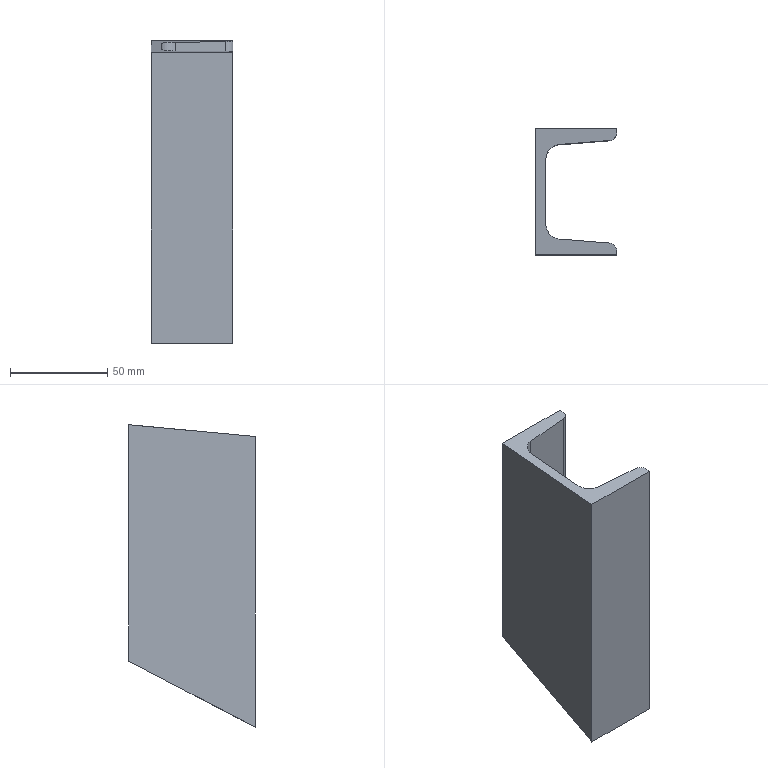Part | STEP file | DIN 1026-1 U 65 1785415623083 | 1 solid | 14 faces | box 42 x 65 x 155.66 mm | volume 122460 mm3 | plane 10 | cylinder 4 | commonest cylinder face diameters 8 x2 15 x2
STEP:
#1=CARTESIAN_POINT('',(42.,30.373,-1.115));
#2=VERTEX_POINT('',#1);
#3=CARTESIAN_POINT('',(42.,32.5,0.));
#4=VERTEX_POINT('',#3);
#5=CARTESIAN_POINT('',(42.,19.754,-6.683));
#6=DIRECTION('',(0.,0.8857,0.4643));
#7=VECTOR('',#6,10.);
#8=LINE('',#5,#7);
#9=EDGE_CURVE('',#2,#4,#8,.T.);
#10=ORIENTED_EDGE('',*,*,#9,.F.);
#11=CARTESIAN_POINT('',(38.319,26.386,-3.206));
#12=VERTEX_POINT('',#11);
#13=CARTESIAN_POINT('',(38.,30.373,-1.115));
#14=DIRECTION('',(0.,-0.4643,0.8857));
#15=DIRECTION('',(0.,0.8857,0.4643));
#16=AXIS2_PLACEMENT_3D('',#13,#14,#15);
#17=ELLIPSE('',#16,4.516,4.);
#18=EDGE_CURVE('',#12,#2,#17,.T.);
#19=ORIENTED_EDGE('',*,*,#18,.F.);
#20=CARTESIAN_POINT('',(12.402,24.312,-4.293));
#21=VERTEX_POINT('',#20);
#22=CARTESIAN_POINT('',(18.401,24.792,-4.041));
#23=DIRECTION('',(0.9959,0.07968,0.04177));
#24=VECTOR('',#23,10.);
#25=LINE('',#22,#24);
#26=EDGE_CURVE('',#21,#12,#25,.T.);
#27=ORIENTED_EDGE('',*,*,#26,.F.);
#28=CARTESIAN_POINT('',(5.5,16.836,-8.212));
#29=VERTEX_POINT('',#28);
#30=CARTESIAN_POINT('',(13.,16.836,-8.212));
#31=DIRECTION('',(0.,0.4643,-0.8857));
#32=DIRECTION('',(0.,0.8857,0.4643));
#33=AXIS2_PLACEMENT_3D('',#30,#31,#32);
#34=ELLIPSE('',#33,8.468,7.5);
#35=EDGE_CURVE('',#29,#21,#34,.T.);
#36=ORIENTED_EDGE('',*,*,#35,.F.);
#37=CARTESIAN_POINT('',(5.5,-16.836,-25.866));
#38=VERTEX_POINT('',#37);
#39=CARTESIAN_POINT('',(5.5,7.007,-13.365));
#40=DIRECTION('',(0.,0.8857,0.4643));
#41=VECTOR('',#40,10.);
#42=LINE('',#39,#41);
#43=EDGE_CURVE('',#38,#29,#42,.T.);
#44=ORIENTED_EDGE('',*,*,#43,.F.);
#45=CARTESIAN_POINT('',(12.402,-24.312,-29.786));
#46=VERTEX_POINT('',#45);
#47=CARTESIAN_POINT('',(13.,-16.836,-25.866));
#48=DIRECTION('',(0.,0.4643,-0.8857));
#49=DIRECTION('',(0.,-0.8857,-0.4643));
#50=AXIS2_PLACEMENT_3D('',#47,#48,#49);
#51=ELLIPSE('',#50,8.468,7.5);
#52=EDGE_CURVE('',#46,#38,#51,.T.);
#53=ORIENTED_EDGE('',*,*,#52,.F.);
#54=CARTESIAN_POINT('',(38.319,-26.386,-30.873));
#55=VERTEX_POINT('',#54);
#56=CARTESIAN_POINT('',(4.047,-23.644,-29.436));
#57=DIRECTION('',(-0.9959,0.07968,0.04177));
#58=VECTOR('',#57,10.);
#59=LINE('',#56,#58);
#60=EDGE_CURVE('',#55,#46,#59,.T.);
#61=ORIENTED_EDGE('',*,*,#60,.F.);
#62=CARTESIAN_POINT('',(42.,-30.373,-32.963));
#63=VERTEX_POINT('',#62);
#64=CARTESIAN_POINT('',(38.,-30.373,-32.963));
#65=DIRECTION('',(0.,-0.4643,0.8857));
#66=DIRECTION('',(0.,-0.8857,-0.4643));
#67=AXIS2_PLACEMENT_3D('',#64,#65,#66);
#68=ELLIPSE('',#67,4.516,4.);
#69=EDGE_CURVE('',#63,#55,#68,.T.);
#70=ORIENTED_EDGE('',*,*,#69,.F.);
#71=CARTESIAN_POINT('',(42.,-32.5,-34.079));
#72=VERTEX_POINT('',#71);
#73=CARTESIAN_POINT('',(42.,-4.905,-19.611));
#74=DIRECTION('',(0.,0.8857,0.4643));
#75=VECTOR('',#74,10.);
#76=LINE('',#73,#75);
#77=EDGE_CURVE('',#72,#63,#76,.T.);
#78=ORIENTED_EDGE('',*,*,#77,.F.);
#79=CARTESIAN_POINT('',(0.,-32.5,-34.079));
#80=VERTEX_POINT('',#79);
#81=CARTESIAN_POINT('',(31.5,-32.5,-34.079));
#82=DIRECTION('',(-1.,0.,0.));
#83=VECTOR('',#82,10.);
#84=LINE('',#81,#83);
#85=EDGE_CURVE('',#72,#80,#84,.T.);
#86=ORIENTED_EDGE('',*,*,#85,.T.);
#87=CARTESIAN_POINT('',(0.,32.5,0.));
#88=VERTEX_POINT('',#87);
#89=CARTESIAN_POINT('',(0.,7.007,-13.365));
#90=DIRECTION('',(0.,-0.8857,-0.4643));
#91=VECTOR('',#90,10.);
#92=LINE('',#89,#91);
#93=EDGE_CURVE('',#88,#80,#92,.T.);
#94=ORIENTED_EDGE('',*,*,#93,.F.);
#95=CARTESIAN_POINT('',(0.,32.5,0.));
#96=DIRECTION('',(-1.,0.,0.));
#97=VECTOR('',#96,10.);
#98=LINE('',#95,#97);
#99=EDGE_CURVE('',#4,#88,#98,.T.);
#100=ORIENTED_EDGE('',*,*,#99,.F.);
#101=EDGE_LOOP('',(#10,#19,#27,#36,#44,#53,#61,#70,#78,#86,#94,#100));
#102=FACE_OUTER_BOUND('',#101,.T.);
#103=CARTESIAN_POINT('',(0.,7.007,-13.365));
#104=DIRECTION('',(0.,-0.4643,0.8857));
#105=DIRECTION('',(1.,0.,0.));
#106=AXIS2_PLACEMENT_3D('',#103,#104,#105);
#107=PLANE('',#106);
#108=ADVANCED_FACE('',(#102),#107,.F.);
#109=ORIENTED_EDGE('',*,*,#60,.T.);
#110=CARTESIAN_POINT('',(12.402,-24.312,116.262));
#111=VERTEX_POINT('',#110);
#112=CARTESIAN_POINT('',(12.402,-24.312,0.));
#113=DIRECTION('',(0.,0.,-1.));
#114=VECTOR('',#113,10.);
#115=LINE('',#112,#114);
#116=EDGE_CURVE('',#111,#46,#115,.T.);
#117=ORIENTED_EDGE('',*,*,#116,.F.);
#118=CARTESIAN_POINT('',(38.319,-26.386,116.068));
#119=VERTEX_POINT('',#118);
#120=CARTESIAN_POINT('',(6.14,-23.811,116.309));
#121=DIRECTION('',(0.9968,-0.07974,-0.007467));
#122=VECTOR('',#121,10.);
#123=LINE('',#120,#122);
#124=EDGE_CURVE('',#111,#119,#123,.T.);
#125=ORIENTED_EDGE('',*,*,#124,.T.);
#126=CARTESIAN_POINT('',(38.319,-26.386,0.));
#127=DIRECTION('',(0.,0.,-1.));
#128=VECTOR('',#127,10.);
#129=LINE('',#126,#128);
#130=EDGE_CURVE('',#119,#55,#129,.T.);
#131=ORIENTED_EDGE('',*,*,#130,.T.);
#132=EDGE_LOOP('',(#109,#117,#125,#131));
#133=FACE_OUTER_BOUND('',#132,.T.);
#134=CARTESIAN_POINT('',(12.402,-24.312,0.));
#135=DIRECTION('',(0.07975,0.9968,0.));
#136=DIRECTION('',(0.,0.,1.));
#137=AXIS2_PLACEMENT_3D('',#134,#135,#136);
#138=PLANE('',#137);
#139=ADVANCED_FACE('',(#133),#138,.T.);
#140=ORIENTED_EDGE('',*,*,#52,.T.);
#141=CARTESIAN_POINT('',(5.5,-16.836,116.962));
#142=VERTEX_POINT('',#141);
#143=CARTESIAN_POINT('',(5.5,-16.836,0.));
#144=DIRECTION('',(0.,0.,-1.));
#145=VECTOR('',#144,10.);
#146=LINE('',#143,#145);
#147=EDGE_CURVE('',#142,#38,#146,.T.);
#148=ORIENTED_EDGE('',*,*,#147,.F.);
#149=CARTESIAN_POINT('',(13.,-16.836,116.962));
#150=DIRECTION('',(0.,-0.09323,0.9956));
#151=DIRECTION('',(0.,-0.9956,-0.09323));
#152=AXIS2_PLACEMENT_3D('',#149,#150,#151);
#153=ELLIPSE('',#152,7.533,7.5);
#154=EDGE_CURVE('',#142,#111,#153,.T.);
#155=ORIENTED_EDGE('',*,*,#154,.T.);
#156=ORIENTED_EDGE('',*,*,#116,.T.);
#157=EDGE_LOOP('',(#140,#148,#155,#156));
#158=FACE_OUTER_BOUND('',#157,.T.);
#159=CARTESIAN_POINT('',(13.,-16.836,0.));
#160=DIRECTION('',(0.,0.,1.));
#161=DIRECTION('',(-1.,0.,0.));
#162=AXIS2_PLACEMENT_3D('',#159,#160,#161);
#163=CYLINDRICAL_SURFACE('',#162,7.5);
#164=ADVANCED_FACE('',(#158),#163,.F.);
#165=ORIENTED_EDGE('',*,*,#43,.T.);
#166=CARTESIAN_POINT('',(5.5,16.836,120.115));
#167=VERTEX_POINT('',#166);
#168=CARTESIAN_POINT('',(5.5,16.836,0.));
#169=DIRECTION('',(0.,0.,-1.));
#170=VECTOR('',#169,10.);
#171=LINE('',#168,#170);
#172=EDGE_CURVE('',#167,#29,#171,.T.);
#173=ORIENTED_EDGE('',*,*,#172,.F.);
#174=CARTESIAN_POINT('',(5.5,-11.004,117.508));
#175=DIRECTION('',(0.,-0.9956,-0.09323));
#176=VECTOR('',#175,10.);
#177=LINE('',#174,#176);
#178=EDGE_CURVE('',#167,#142,#177,.T.);
#179=ORIENTED_EDGE('',*,*,#178,.T.);
#180=ORIENTED_EDGE('',*,*,#147,.T.);
#181=EDGE_LOOP('',(#165,#173,#179,#180));
#182=FACE_OUTER_BOUND('',#181,.T.);
#183=CARTESIAN_POINT('',(5.5,0.,0.));
#184=DIRECTION('',(1.,0.,0.));
#185=DIRECTION('',(0.,0.,-1.));
#186=AXIS2_PLACEMENT_3D('',#183,#184,#185);
#187=PLANE('',#186);
#188=ADVANCED_FACE('',(#182),#187,.T.);
#189=ORIENTED_EDGE('',*,*,#35,.T.);
#190=CARTESIAN_POINT('',(12.402,24.312,120.815));
#191=VERTEX_POINT('',#190);
#192=CARTESIAN_POINT('',(12.402,24.312,0.));
#193=DIRECTION('',(0.,0.,-1.));
#194=VECTOR('',#193,10.);
#195=LINE('',#192,#194);
#196=EDGE_CURVE('',#191,#21,#195,.T.);
#197=ORIENTED_EDGE('',*,*,#196,.F.);
#198=CARTESIAN_POINT('',(13.,16.836,120.115));
#199=DIRECTION('',(0.,-0.09323,0.9956));
#200=DIRECTION('',(0.,0.9956,0.09323));
#201=AXIS2_PLACEMENT_3D('',#198,#199,#200);
#202=ELLIPSE('',#201,7.533,7.5);
#203=EDGE_CURVE('',#191,#167,#202,.T.);
#204=ORIENTED_EDGE('',*,*,#203,.T.);
#205=ORIENTED_EDGE('',*,*,#172,.T.);
#206=EDGE_LOOP('',(#189,#197,#204,#205));
#207=FACE_OUTER_BOUND('',#206,.T.);
#208=CARTESIAN_POINT('',(13.,16.836,0.));
#209=DIRECTION('',(0.,0.,1.));
#210=DIRECTION('',(-0.07975,0.9968,0.));
#211=AXIS2_PLACEMENT_3D('',#208,#209,#210);
#212=CYLINDRICAL_SURFACE('',#211,7.5);
#213=ADVANCED_FACE('',(#207),#212,.F.);
#214=ORIENTED_EDGE('',*,*,#26,.T.);
#215=CARTESIAN_POINT('',(38.319,26.386,121.009));
#216=VERTEX_POINT('',#215);
#217=CARTESIAN_POINT('',(38.319,26.386,0.));
#218=DIRECTION('',(0.,0.,-1.));
#219=VECTOR('',#218,10.);
#220=LINE('',#217,#219);
#221=EDGE_CURVE('',#216,#12,#220,.T.);
#222=ORIENTED_EDGE('',*,*,#221,.F.);
#223=CARTESIAN_POINT('',(17.333,24.707,120.852));
#224=DIRECTION('',(-0.9968,-0.07974,-0.007467));
#225=VECTOR('',#224,10.);
#226=LINE('',#223,#225);
#227=EDGE_CURVE('',#216,#191,#226,.T.);
#228=ORIENTED_EDGE('',*,*,#227,.T.);
#229=ORIENTED_EDGE('',*,*,#196,.T.);
#230=EDGE_LOOP('',(#214,#222,#228,#229));
#231=FACE_OUTER_BOUND('',#230,.T.);
#232=CARTESIAN_POINT('',(38.319,26.386,0.));
#233=DIRECTION('',(0.07975,-0.9968,0.));
#234=DIRECTION('',(0.,0.,-1.));
#235=AXIS2_PLACEMENT_3D('',#232,#233,#234);
#236=PLANE('',#235);
#237=ADVANCED_FACE('',(#231),#236,.T.);
#238=ORIENTED_EDGE('',*,*,#18,.T.);
#239=CARTESIAN_POINT('',(42.,30.373,121.383));
#240=VERTEX_POINT('',#239);
#241=CARTESIAN_POINT('',(42.,30.373,0.));
#242=DIRECTION('',(0.,0.,-1.));
#243=VECTOR('',#242,10.);
#244=LINE('',#241,#243);
#245=EDGE_CURVE('',#240,#2,#244,.T.);
#246=ORIENTED_EDGE('',*,*,#245,.F.);
#247=CARTESIAN_POINT('',(38.,30.373,121.383));
#248=DIRECTION('',(0.,0.09323,-0.9956));
#249=DIRECTION('',(0.,0.9956,0.09323));
#250=AXIS2_PLACEMENT_3D('',#247,#248,#249);
#251=ELLIPSE('',#250,4.017,4.);
#252=EDGE_CURVE('',#240,#216,#251,.T.);
#253=ORIENTED_EDGE('',*,*,#252,.T.);
#254=ORIENTED_EDGE('',*,*,#221,.T.);
#255=EDGE_LOOP('',(#238,#246,#253,#254));
#256=FACE_OUTER_BOUND('',#255,.T.);
#257=CARTESIAN_POINT('',(38.,30.373,0.));
#258=DIRECTION('',(0.,0.,1.));
#259=DIRECTION('',(-0.07975,0.9968,0.));
#260=AXIS2_PLACEMENT_3D('',#257,#258,#259);
#261=CYLINDRICAL_SURFACE('',#260,4.);
#262=ADVANCED_FACE('',(#256),#261,.T.);
#263=ORIENTED_EDGE('',*,*,#154,.F.);
#264=ORIENTED_EDGE('',*,*,#178,.F.);
#265=ORIENTED_EDGE('',*,*,#203,.F.);
#266=ORIENTED_EDGE('',*,*,#227,.F.);
#267=ORIENTED_EDGE('',*,*,#252,.F.);
#268=CARTESIAN_POINT('',(42.,32.5,121.582));
#269=VERTEX_POINT('',#268);
#270=CARTESIAN_POINT('',(42.,5.105,119.016));
#271=DIRECTION('',(0.,-0.9956,-0.09323));
#272=VECTOR('',#271,10.);
#273=LINE('',#270,#272);
#274=EDGE_CURVE('',#269,#240,#273,.T.);
#275=ORIENTED_EDGE('',*,*,#274,.F.);
#276=CARTESIAN_POINT('',(0.,32.5,121.582));
#277=VERTEX_POINT('',#276);
#278=CARTESIAN_POINT('',(10.5,32.5,121.582));
#279=DIRECTION('',(1.,0.,0.));
#280=VECTOR('',#279,10.);
#281=LINE('',#278,#280);
#282=EDGE_CURVE('',#277,#269,#281,.T.);
#283=ORIENTED_EDGE('',*,*,#282,.F.);
#284=CARTESIAN_POINT('',(0.,-32.5,115.495));
#285=VERTEX_POINT('',#284);
#286=CARTESIAN_POINT('',(0.,-11.004,117.508));
#287=DIRECTION('',(0.,0.9956,0.09323));
#288=VECTOR('',#287,10.);
#289=LINE('',#286,#288);
#290=EDGE_CURVE('',#285,#277,#289,.T.);
#291=ORIENTED_EDGE('',*,*,#290,.F.);
#292=CARTESIAN_POINT('',(42.,-32.5,115.495));
#293=VERTEX_POINT('',#292);
#294=CARTESIAN_POINT('',(21.,-32.5,115.495));
#295=DIRECTION('',(-1.,0.,0.));
#296=VECTOR('',#295,10.);
#297=LINE('',#294,#296);
#298=EDGE_CURVE('',#293,#285,#297,.T.);
#299=ORIENTED_EDGE('',*,*,#298,.F.);
#300=CARTESIAN_POINT('',(42.,-30.373,115.694));
#301=VERTEX_POINT('',#300);
#302=CARTESIAN_POINT('',(42.,-26.058,116.098));
#303=DIRECTION('',(0.,-0.9956,-0.09323));
#304=VECTOR('',#303,10.);
#305=LINE('',#302,#304);
#306=EDGE_CURVE('',#301,#293,#305,.T.);
#307=ORIENTED_EDGE('',*,*,#306,.F.);
#308=CARTESIAN_POINT('',(38.,-30.373,115.694));
#309=DIRECTION('',(0.,0.09323,-0.9956));
#310=DIRECTION('',(0.,-0.9956,-0.09323));
#311=AXIS2_PLACEMENT_3D('',#308,#309,#310);
#312=ELLIPSE('',#311,4.017,4.);
#313=EDGE_CURVE('',#119,#301,#312,.T.);
#314=ORIENTED_EDGE('',*,*,#313,.F.);
#315=ORIENTED_EDGE('',*,*,#124,.F.);
#316=EDGE_LOOP('',(#263,#264,#265,#266,#267,#275,#283,#291,#299,#307,#314,#315));
#317=FACE_OUTER_BOUND('',#316,.T.);
#318=CARTESIAN_POINT('',(0.,-11.004,117.508));
#319=DIRECTION('',(0.,0.09323,-0.9956));
#320=DIRECTION('',(-1.,0.,0.));
#321=AXIS2_PLACEMENT_3D('',#318,#319,#320);
#322=PLANE('',#321);
#323=ADVANCED_FACE('',(#317),#322,.F.);
#324=ORIENTED_EDGE('',*,*,#9,.T.);
#325=CARTESIAN_POINT('',(42.,32.5,0.));
#326=DIRECTION('',(0.,0.,-1.));
#327=VECTOR('',#326,10.);
#328=LINE('',#325,#327);
#329=EDGE_CURVE('',#269,#4,#328,.T.);
#330=ORIENTED_EDGE('',*,*,#329,.F.);
#331=ORIENTED_EDGE('',*,*,#274,.T.);
#332=ORIENTED_EDGE('',*,*,#245,.T.);
#333=EDGE_LOOP('',(#324,#330,#331,#332));
#334=FACE_OUTER_BOUND('',#333,.T.);
#335=CARTESIAN_POINT('',(42.,32.5,0.));
#336=DIRECTION('',(1.,0.,0.));
#337=DIRECTION('',(0.,0.,-1.));
#338=AXIS2_PLACEMENT_3D('',#335,#336,#337);
#339=PLANE('',#338);
#340=ADVANCED_FACE('',(#334),#339,.T.);
#341=ORIENTED_EDGE('',*,*,#69,.T.);
#342=ORIENTED_EDGE('',*,*,#130,.F.);
#343=ORIENTED_EDGE('',*,*,#313,.T.);
#344=CARTESIAN_POINT('',(42.,-30.373,0.));
#345=DIRECTION('',(0.,0.,-1.));
#346=VECTOR('',#345,10.);
#347=LINE('',#344,#346);
#348=EDGE_CURVE('',#301,#63,#347,.T.);
#349=ORIENTED_EDGE('',*,*,#348,.T.);
#350=EDGE_LOOP('',(#341,#342,#343,#349));
#351=FACE_OUTER_BOUND('',#350,.T.);
#352=CARTESIAN_POINT('',(38.,-30.373,0.));
#353=DIRECTION('',(0.,0.,1.));
#354=DIRECTION('',(-1.,0.,0.));
#355=AXIS2_PLACEMENT_3D('',#352,#353,#354);
#356=CYLINDRICAL_SURFACE('',#355,4.);
#357=ADVANCED_FACE('',(#351),#356,.T.);
#358=ORIENTED_EDGE('',*,*,#77,.T.);
#359=ORIENTED_EDGE('',*,*,#348,.F.);
#360=ORIENTED_EDGE('',*,*,#306,.T.);
#361=CARTESIAN_POINT('',(42.,-32.5,0.));
#362=DIRECTION('',(0.,0.,-1.));
#363=VECTOR('',#362,10.);
#364=LINE('',#361,#363);
#365=EDGE_CURVE('',#293,#72,#364,.T.);
#366=ORIENTED_EDGE('',*,*,#365,.T.);
#367=EDGE_LOOP('',(#358,#359,#360,#366));
#368=FACE_OUTER_BOUND('',#367,.T.);
#369=CARTESIAN_POINT('',(42.,-30.373,0.));
#370=DIRECTION('',(1.,0.,0.));
#371=DIRECTION('',(0.,0.,-1.));
#372=AXIS2_PLACEMENT_3D('',#369,#370,#371);
#373=PLANE('',#372);
#374=ADVANCED_FACE('',(#368),#373,.T.);
#375=ORIENTED_EDGE('',*,*,#298,.T.);
#376=CARTESIAN_POINT('',(0.,-32.5,0.));
#377=DIRECTION('',(0.,0.,-1.));
#378=VECTOR('',#377,10.);
#379=LINE('',#376,#378);
#380=EDGE_CURVE('',#285,#80,#379,.T.);
#381=ORIENTED_EDGE('',*,*,#380,.T.);
#382=ORIENTED_EDGE('',*,*,#85,.F.);
#383=ORIENTED_EDGE('',*,*,#365,.F.);
#384=EDGE_LOOP('',(#375,#381,#382,#383));
#385=FACE_OUTER_BOUND('',#384,.T.);
#386=CARTESIAN_POINT('',(42.,-32.5,0.));
#387=DIRECTION('',(0.,-1.,0.));
#388=DIRECTION('',(0.,0.,-1.));
#389=AXIS2_PLACEMENT_3D('',#386,#387,#388);
#390=PLANE('',#389);
#391=ADVANCED_FACE('',(#385),#390,.T.);
#392=ORIENTED_EDGE('',*,*,#93,.T.);
#393=ORIENTED_EDGE('',*,*,#380,.F.);
#394=ORIENTED_EDGE('',*,*,#290,.T.);
#395=CARTESIAN_POINT('',(0.,32.5,0.));
#396=DIRECTION('',(0.,0.,-1.));
#397=VECTOR('',#396,10.);
#398=LINE('',#395,#397);
#399=EDGE_CURVE('',#277,#88,#398,.T.);
#400=ORIENTED_EDGE('',*,*,#399,.T.);
#401=EDGE_LOOP('',(#392,#393,#394,#400));
#402=FACE_OUTER_BOUND('',#401,.T.);
#403=CARTESIAN_POINT('',(0.,0.,0.));
#404=DIRECTION('',(-1.,0.,0.));
#405=DIRECTION('',(0.,0.,1.));
#406=AXIS2_PLACEMENT_3D('',#403,#404,#405);
#407=PLANE('',#406);
#408=ADVANCED_FACE('',(#402),#407,.T.);
#409=ORIENTED_EDGE('',*,*,#99,.T.);
#410=ORIENTED_EDGE('',*,*,#399,.F.);
#411=ORIENTED_EDGE('',*,*,#282,.T.);
#412=ORIENTED_EDGE('',*,*,#329,.T.);
#413=EDGE_LOOP('',(#409,#410,#411,#412));
#414=FACE_OUTER_BOUND('',#413,.T.);
#415=CARTESIAN_POINT('',(0.,32.5,0.));
#416=DIRECTION('',(0.,1.,0.));
#417=DIRECTION('',(0.,0.,1.));
#418=AXIS2_PLACEMENT_3D('',#415,#416,#417);
#419=PLANE('',#418);
#420=ADVANCED_FACE('',(#414),#419,.T.);
#421=CLOSED_SHELL('',(#108,#139,#164,#188,#213,#237,#262,#323,#340,#357,#374,#391,#408,#420));
#422=MANIFOLD_SOLID_BREP('',#421);
#423=(LENGTH_UNIT()NAMED_UNIT(*)SI_UNIT(.MILLI.,.METRE.));
#424=UNCERTAINTY_MEASURE_WITH_UNIT(LENGTH_MEASURE(0.01),#423,'','');
#425=(NAMED_UNIT(*)PLANE_ANGLE_UNIT()SI_UNIT($,.RADIAN.));
#426=(NAMED_UNIT(*)SI_UNIT($,.STERADIAN.)SOLID_ANGLE_UNIT());
#427=(GEOMETRIC_REPRESENTATION_CONTEXT(3)GLOBAL_UNCERTAINTY_ASSIGNED_CONTEXT((#424))GLOBAL_UNIT_ASSIGNED_CONTEXT((#423,#425,#426))REPRESENTATION_CONTEXT('',''));
#428=ADVANCED_BREP_SHAPE_REPRESENTATION('',(#422),#427);